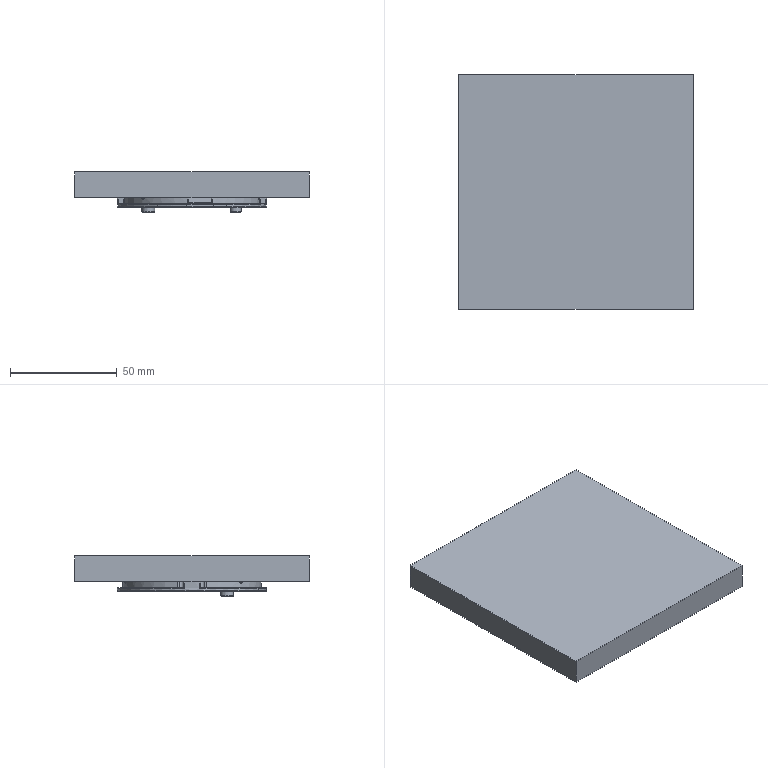NC program | NX | posted with a generic post | part box 110 x 110 x 18.8 mm
Lines 1770 to 3401 of 9447, first 1467 of 1628 lines:
(CAVITY_MILL_COPY_1 , TOOL : D6)
N3532 T16 M6
N3534 G54
N3536 G17 G0 G90 X7.71 Y22.388 S9500 M3
N3538 G43 Z30. H16
N3540 Z-4.5
N3542 G94 G1 Z-5.5 F1000.
N3544 X8.202 Y21.964
N3546 G3 X9.184 Y21.777 R1.
N3548 G2 X10.5 Y22. R4. F1600.
N3550 G1 X16.333
N3552 G3 X9.42 Y25.73 R27.4
N3554 X8.435 Y25.558 R1.
N3556 G1 X7.786 Y25.016
N3558 Z-4.5
N3560 G0 X7.71 Y22.388 Z-5.
N3562 G1 Z-6. F1000.
N3564 X8.202 Y21.964
N3566 G3 X9.184 Y21.777 R1.
N3568 G2 X10.5 Y22. R4. F1600.
N3570 G1 X16.333
N3572 G3 X9.42 Y25.73 R27.4
N3574 X8.435 Y25.558 R1.
N3576 G1 X7.786 Y25.016
N3578 Z-5.
N3580 G0 X7.71 Y22.388 Z-5.5
N3582 G1 Z-6.5 F1000.
N3584 X8.202 Y21.964
N3586 G3 X9.184 Y21.777 R1.
N3588 G2 X10.5 Y22. R4. F1600.
N3590 G1 X16.333
N3592 G3 X9.42 Y25.73 R27.4
N3594 X8.435 Y25.558 R1.
N3596 G1 X7.786 Y25.016
N3598 Z-5.5
N3600 G0 X7.71 Y22.388 Z-6.
N3602 G1 Z-7. F1000.
N3604 X8.202 Y21.964
N3606 G3 X9.184 Y21.777 R1.
N3608 G2 X10.5 Y22. R4. F1600.
N3610 G1 X16.333
N3612 G3 X9.42 Y25.73 R27.4
N3614 X8.435 Y25.558 R1.
N3616 G1 X7.786 Y25.016
N3618 Z-6.
N3620 G0 X7.71 Y22.388 Z-6.5
N3622 G1 Z-7.5 F1000.
N3624 X8.202 Y21.964
N3626 G3 X9.184 Y21.777 R1.
N3628 G2 X10.5 Y22. R4. F1600.
N3630 G1 X16.333
N3632 G3 X9.42 Y25.73 R27.4
N3634 X8.435 Y25.558 R1.
N3636 G1 X7.786 Y25.016
N3638 Z-6.5
N3640 G0 X7.71 Y22.388 Z-7.
N3642 G1 Z-8. F1000.
N3644 X8.202 Y21.964
N3646 G3 X9.184 Y21.777 R1.
N3648 G2 X10.5 Y22. R4. F1600.
N3650 G1 X16.333
N3652 G3 X9.42 Y25.73 R27.4
N3654 X8.435 Y25.558 R1.
N3656 G1 X7.786 Y25.016
N3658 Z-7.
N3660 G0 X7.71 Y22.388 Z-7.5
N3662 G1 Z-8.5 F1000.
N3664 X8.202 Y21.964
N3666 G3 X9.184 Y21.777 R1.
N3668 G2 X10.5 Y22. R4. F1600.
N3670 G1 X16.333
N3672 G3 X9.42 Y25.73 R27.4
N3674 X8.435 Y25.558 R1.
N3676 G1 X7.786 Y25.016
N3678 Z-7.5
N3680 G0 X7.71 Y22.388 Z-8.
N3682 G1 Z-9. F1000.
N3684 X8.202 Y21.964
N3686 G3 X9.184 Y21.777 R1.
N3688 G2 X10.5 Y22. R4. F1600.
N3690 G1 X16.333
N3692 G3 X9.42 Y25.73 R27.4
N3694 X8.435 Y25.558 R1.
N3696 G1 X7.786 Y25.016
N3698 Z-8.
N3700 G0 X7.71 Y22.388 Z-8.5
N3702 G1 Z-9.5 F1000.
N3704 X8.202 Y21.964
N3706 G3 X9.184 Y21.777 R1.
N3708 G2 X10.5 Y22. R4. F1600.
N3710 G1 X16.333
N3712 G3 X9.42 Y25.73 R27.4
N3714 X8.435 Y25.558 R1.
N3716 G1 X7.786 Y25.016
N3718 Z-8.5
N3720 G0 X7.71 Y22.388 Z-9.
N3722 G1 Z-10. F1000.
N3724 X8.202 Y21.964
N3726 G3 X9.184 Y21.777 R1.
N3728 G2 X10.5 Y22. R4. F1600.
N3730 G1 X16.333
N3732 G3 X9.42 Y25.73 R27.4
N3734 X8.435 Y25.558 R1.
N3736 G1 X7.786 Y25.016
N3738 Z-9.
N3740 G0 X7.71 Y22.388 Z-9.5
N3742 G1 Z-10.5 F1000.
N3744 X8.202 Y21.964
N3746 G3 X9.184 Y21.777 R1.
N3748 G2 X10.5 Y22. R4. F1600.
N3750 G1 X16.333
N3752 G3 X9.42 Y25.73 R27.4
N3754 X8.435 Y25.558 R1.
N3756 G1 X7.786 Y25.016
N3758 Z-9.5
N3760 G0 X7.71 Y22.388 Z-10.
N3762 G1 Z-11. F1000.
N3764 X8.202 Y21.964
N3766 G3 X9.184 Y21.777 R1.
N3768 G2 X10.5 Y22. R4. F1600.
N3770 G1 X16.333
N3772 G3 X9.42 Y25.73 R27.4
N3774 X8.435 Y25.558 R1.
N3776 G1 X7.786 Y25.016
N3778 Z-10.
N3780 G0 X7.71 Y22.388 Z-10.5
N3782 G1 Z-11.5 F1000.
N3784 X8.202 Y21.964
N3786 G3 X9.184 Y21.777 R1.
N3788 G2 X10.5 Y22. R4. F1600.
N3790 G1 X16.333
N3792 G3 X9.42 Y25.73 R27.4
N3794 X8.435 Y25.558 R1.
N3796 G1 X7.786 Y25.016
N3798 Z-10.5
N3800 G0 Z30.
N3802 X26.5 Y2.101
N3804 Z2.
N3806 G1 Y-1.733 Z1.799 F1000.
N3808 X26.714 Y-1.548 Z1.784
N3810 X27.121 Y-1.282 Z1.759
N3812 X27.375 Y-1.159 Z1.744
N3814 X27.407 Y-0.419 Z1.705
N3816 X27.381 Y1.261 Z1.617
N3818 X27.252 Y2.937 Z1.529
N3820 X27.021 Y4.602 Z1.441
N3822 X26.688 Y6.249 Z1.353
N3824 X26.5 Y6.965 Z1.314
N3826 Y-1.733 Z0.858
N3828 X26.714 Y-1.548 Z0.843
N3830 X27.121 Y-1.282 Z0.818
N3832 X27.375 Y-1.159 Z0.803
N3834 X27.407 Y-0.419 Z0.764
N3836 X27.381 Y1.261 Z0.676
N3838 X27.252 Y2.937 Z0.588
N3840 X27.021 Y4.602 Z0.5
N3842 X26.688 Y6.249 Z0.412
N3844 X26.5 Y6.965 Z0.373
N3846 Y-1.733 Z-0.083
N3848 X26.714 Y-1.548 Z-0.098
N3850 X27.121 Y-1.282 Z-0.123
N3852 X27.375 Y-1.159 Z-0.138
N3854 X27.407 Y-0.419 Z-0.177
N3856 X27.381 Y1.261 Z-0.265
N3858 X27.252 Y2.937 Z-0.353
N3860 X27.021 Y4.602 Z-0.441
N3862 X26.688 Y6.249 Z-0.529
N3864 X26.5 Y6.965 Z-0.568
N3866 Y-1.733 Z-1.024
N3868 X26.714 Y-1.548 Z-1.038
N3870 X27.121 Y-1.282 Z-1.064
N3872 X27.375 Y-1.159 Z-1.079
N3874 X27.407 Y-0.419 Z-1.117
N3876 X27.381 Y1.261 Z-1.206
N3878 X27.252 Y2.937 Z-1.294
N3880 X27.021 Y4.602 Z-1.382
N3882 X26.688 Y6.249 Z-1.47
N3884 X26.5 Y6.965 Z-1.509
N3886 Y-1.733 Z-1.964
N3888 X26.714 Y-1.548 Z-1.979
N3890 X27.121 Y-1.282 Z-2.005
N3892 X27.375 Y-1.159 Z-2.02
N3894 X27.407 Y-0.419 Z-2.058
N3896 X27.381 Y1.261 Z-2.146
N3898 X27.252 Y2.937 Z-2.235
N3900 X27.021 Y4.602 Z-2.323
N3902 X26.688 Y6.249 Z-2.411
N3904 X26.5 Y6.965 Z-2.449
N3906 Y-1.733 Z-2.905
N3908 X26.714 Y-1.548 Z-2.92
N3910 X27.121 Y-1.282 Z-2.946
N3912 X27.375 Y-1.159 Z-2.96
N3914 X27.407 Y-0.419 Z-2.999
N3916 X27.381 Y1.261 Z-3.087
N3918 X27.252 Y2.937 Z-3.175
N3920 X27.021 Y4.602 Z-3.263
N3922 X26.688 Y6.249 Z-3.352
N3924 X26.5 Y6.965 Z-3.39
N3926 Y-1.733 Z-3.846
N3928 X26.714 Y-1.548 Z-3.861
N3930 X27.121 Y-1.282 Z-3.886
N3932 X27.375 Y-1.159 Z-3.901
N3934 X27.407 Y-0.419 Z-3.94
N3936 X27.381 Y1.261 Z-4.028
N3938 X27.252 Y2.937 Z-4.116
N3940 X27.021 Y4.602 Z-4.204
N3942 X26.688 Y6.249 Z-4.292
N3944 X26.5 Y6.965 Z-4.331
N3946 Y-1.733 Z-4.787
N3948 X26.714 Y-1.548 Z-4.802
N3950 X27.121 Y-1.282 Z-4.827
N3952 X27.375 Y-1.159 Z-4.842
N3954 X27.407 Y-0.419 Z-4.881
N3956 X27.381 Y1.261 Z-4.969
N3958 X27.252 Y2.937 Z-5.057
N3960 X27.021 Y4.602 Z-5.145
N3962 X26.688 Y6.249 Z-5.233
N3964 X26.5 Y6.965 Z-5.272
N3966 Y2.616 Z-5.5
N3968 Y-1.733 F1600.
N3970 G2 X27.375 Y-1.159 R4.
N3972 G3 X26.5 Y6.965 R27.4
N3974 G1 Y2.616
N3976 G3 X27. Y1.75 R1.
N3978 G1 Z-4.5
N3980 G0 X27.389 Y0.724
N3982 G1 X27.381 Y1.261 Z-4.528 F1000.
N3984 X27.252 Y2.937 Z-4.616
N3986 X27.021 Y4.602 Z-4.704
N3988 X26.688 Y6.249 Z-4.792
N3990 X26.5 Y6.965 Z-4.831
N3992 Y-1.733 Z-5.287
N3994 X26.714 Y-1.548 Z-5.302
N3996 X27.121 Y-1.282 Z-5.327
N3998 X27.375 Y-1.159 Z-5.342
N4000 X27.407 Y-0.419 Z-5.381
N4002 X27.381 Y1.261 Z-5.469
N4004 X27.252 Y2.937 Z-5.557
N4006 X27.021 Y4.602 Z-5.645
N4008 X26.688 Y6.249 Z-5.733
N4010 X26.5 Y6.965 Z-5.772
N4012 Y2.616 Z-6.
N4014 Y-1.733 F1600.
N4016 G2 X27.375 Y-1.159 R4.
N4018 G3 X26.5 Y6.965 R27.4
N4020 G1 Y2.616
N4022 G3 X27. Y1.75 R1.
N4024 G1 Z-5.
N4026 G0 X27.389 Y0.724
N4028 G1 X27.381 Y1.261 Z-5.028 F1000.
N4030 X27.252 Y2.937 Z-5.116
N4032 X27.021 Y4.602 Z-5.204
N4034 X26.688 Y6.249 Z-5.292
N4036 X26.5 Y6.965 Z-5.331
N4038 Y-1.733 Z-5.787
N4040 X26.714 Y-1.548 Z-5.802
N4042 X27.121 Y-1.282 Z-5.827
N4044 X27.375 Y-1.159 Z-5.842
N4046 X27.407 Y-0.419 Z-5.881
N4048 X27.381 Y1.261 Z-5.969
N4050 X27.252 Y2.937 Z-6.057
N4052 X27.021 Y4.602 Z-6.145
N4054 X26.688 Y6.249 Z-6.233
N4056 X26.5 Y6.965 Z-6.272
N4058 Y2.616 Z-6.5
N4060 Y-1.733 F1600.
N4062 G2 X27.375 Y-1.159 R4.
N4064 G3 X26.5 Y6.965 R27.4
N4066 G1 Y2.616
N4068 G3 X27. Y1.75 R1.
N4070 G1 Z-5.5
N4072 G0 X27.389 Y0.724
N4074 G1 X27.381 Y1.261 Z-5.528 F1000.
N4076 X27.252 Y2.937 Z-5.616
N4078 X27.021 Y4.602 Z-5.704
N4080 X26.688 Y6.249 Z-5.792
N4082 X26.5 Y6.965 Z-5.831
N4084 Y-1.733 Z-6.287
N4086 X26.714 Y-1.548 Z-6.302
N4088 X27.121 Y-1.282 Z-6.327
N4090 X27.375 Y-1.159 Z-6.342
N4092 X27.407 Y-0.419 Z-6.381
N4094 X27.381 Y1.261 Z-6.469
N4096 X27.252 Y2.937 Z-6.557
N4098 X27.021 Y4.602 Z-6.645
N4100 X26.688 Y6.249 Z-6.733
N4102 X26.5 Y6.965 Z-6.772
N4104 Y2.616 Z-7.
N4106 Y-1.733 F1600.
N4108 G2 X27.375 Y-1.159 R4.
N4110 G3 X26.5 Y6.965 R27.4
N4112 G1 Y2.616
N4114 G3 X27. Y1.75 R1.
N4116 G1 Z-6.
N4118 G0 X27.389 Y0.724
N4120 G1 X27.381 Y1.261 Z-6.028 F1000.
N4122 X27.252 Y2.937 Z-6.116
N4124 X27.021 Y4.602 Z-6.204
N4126 X26.688 Y6.249 Z-6.292
N4128 X26.5 Y6.965 Z-6.331
N4130 Y-1.733 Z-6.787
N4132 X26.714 Y-1.548 Z-6.802
N4134 X27.121 Y-1.282 Z-6.827
N4136 X27.375 Y-1.159 Z-6.842
N4138 X27.407 Y-0.419 Z-6.881
N4140 X27.381 Y1.261 Z-6.969
N4142 X27.252 Y2.937 Z-7.057
N4144 X27.021 Y4.602 Z-7.145
N4146 X26.688 Y6.249 Z-7.233
N4148 X26.5 Y6.965 Z-7.272
N4150 Y2.616 Z-7.5
N4152 Y-1.733 F1600.
N4154 G2 X27.375 Y-1.159 R4.
N4156 G3 X26.5 Y6.965 R27.4
N4158 G1 Y2.616
N4160 G3 X27. Y1.75 R1.
N4162 G1 Z-6.5
N4164 G0 X27.389 Y0.724
N4166 G1 X27.381 Y1.261 Z-6.528 F1000.
N4168 X27.252 Y2.937 Z-6.616
N4170 X27.021 Y4.602 Z-6.704
N4172 X26.688 Y6.249 Z-6.792
N4174 X26.5 Y6.965 Z-6.831
N4176 Y-1.733 Z-7.287
N4178 X26.714 Y-1.548 Z-7.302
N4180 X27.121 Y-1.282 Z-7.327
N4182 X27.375 Y-1.159 Z-7.342
N4184 X27.407 Y-0.419 Z-7.381
N4186 X27.381 Y1.261 Z-7.469
N4188 X27.252 Y2.937 Z-7.557
N4190 X27.021 Y4.602 Z-7.645
N4192 X26.688 Y6.249 Z-7.733
N4194 X26.5 Y6.965 Z-7.772
N4196 Y2.616 Z-8.
N4198 Y-1.733 F1600.
N4200 G2 X27.375 Y-1.159 R4.
N4202 G3 X26.5 Y6.965 R27.4
N4204 G1 Y2.616
N4206 G3 X27. Y1.75 R1.
N4208 G1 Z-7.
N4210 G0 X27.389 Y0.724
N4212 G1 X27.381 Y1.261 Z-7.028 F1000.
N4214 X27.252 Y2.937 Z-7.116
N4216 X27.021 Y4.602 Z-7.204
N4218 X26.688 Y6.249 Z-7.292
N4220 X26.5 Y6.965 Z-7.331
N4222 Y-1.733 Z-7.787
N4224 X26.714 Y-1.548 Z-7.802
N4226 X27.121 Y-1.282 Z-7.827
N4228 X27.375 Y-1.159 Z-7.842
N4230 X27.407 Y-0.419 Z-7.881
N4232 X27.381 Y1.261 Z-7.969
N4234 X27.252 Y2.937 Z-8.057
N4236 X27.021 Y4.602 Z-8.145
N4238 X26.688 Y6.249 Z-8.233
N4240 X26.5 Y6.965 Z-8.272
N4242 Y2.616 Z-8.5
N4244 Y-1.733 F1600.
N4246 G2 X27.375 Y-1.159 R4.
N4248 G3 X26.5 Y6.965 R27.4
N4250 G1 Y2.616
N4252 G3 X27. Y1.75 R1.
N4254 G1 Z-7.5
N4256 G0 X27.389 Y0.724
N4258 G1 X27.381 Y1.261 Z-7.528 F1000.
N4260 X27.252 Y2.937 Z-7.616
N4262 X27.021 Y4.602 Z-7.704
N4264 X26.688 Y6.249 Z-7.792
N4266 X26.5 Y6.965 Z-7.831
N4268 Y-1.733 Z-8.287
N4270 X26.714 Y-1.548 Z-8.302
N4272 X27.121 Y-1.282 Z-8.327
N4274 X27.375 Y-1.159 Z-8.342
N4276 X27.407 Y-0.419 Z-8.381
N4278 X27.381 Y1.261 Z-8.469
N4280 X27.252 Y2.937 Z-8.557
N4282 X27.021 Y4.602 Z-8.645
N4284 X26.688 Y6.249 Z-8.733
N4286 X26.5 Y6.965 Z-8.772
N4288 Y2.616 Z-9.
N4290 Y-1.733 F1600.
N4292 G2 X27.375 Y-1.159 R4.
N4294 G3 X26.5 Y6.965 R27.4
N4296 G1 Y2.616
N4298 G3 X27. Y1.75 R1.
N4300 G1 Z-8.
N4302 G0 X27.389 Y0.724
N4304 G1 X27.381 Y1.261 Z-8.028 F1000.
N4306 X27.252 Y2.937 Z-8.116
N4308 X27.021 Y4.602 Z-8.204
N4310 X26.688 Y6.249 Z-8.292
N4312 X26.5 Y6.965 Z-8.331
N4314 Y-1.733 Z-8.787
N4316 X26.714 Y-1.548 Z-8.802
N4318 X27.121 Y-1.282 Z-8.827
N4320 X27.375 Y-1.159 Z-8.842
N4322 X27.407 Y-0.419 Z-8.881
N4324 X27.381 Y1.261 Z-8.969
N4326 X27.252 Y2.937 Z-9.057
N4328 X27.021 Y4.602 Z-9.145
N4330 X26.688 Y6.249 Z-9.233
N4332 X26.5 Y6.965 Z-9.272
N4334 Y2.616 Z-9.5
N4336 Y-1.733 F1600.
N4338 G2 X27.375 Y-1.159 R4.
N4340 G3 X26.5 Y6.965 R27.4
N4342 G1 Y2.616
N4344 G3 X27. Y1.75 R1.
N4346 G1 Z-8.5
N4348 G0 X27.389 Y0.724
N4350 G1 X27.381 Y1.261 Z-8.528 F1000.
N4352 X27.252 Y2.937 Z-8.616
N4354 X27.021 Y4.602 Z-8.704
N4356 X26.688 Y6.249 Z-8.792
N4358 X26.5 Y6.965 Z-8.831
N4360 Y-1.733 Z-9.287
N4362 X26.714 Y-1.548 Z-9.302
N4364 X27.121 Y-1.282 Z-9.327
N4366 X27.375 Y-1.159 Z-9.342
N4368 X27.407 Y-0.419 Z-9.381
N4370 X27.381 Y1.261 Z-9.469
N4372 X27.252 Y2.937 Z-9.557
N4374 X27.021 Y4.602 Z-9.645
N4376 X26.688 Y6.249 Z-9.733
N4378 X26.5 Y6.965 Z-9.772
N4380 Y2.616 Z-10.
N4382 Y-1.733 F1600.
N4384 G2 X27.375 Y-1.159 R4.
N4386 G3 X26.5 Y6.965 R27.4
N4388 G1 Y2.616
N4390 G3 X27. Y1.75 R1.
N4392 G1 Z-9.
N4394 G0 X27.389 Y0.724
N4396 G1 X27.381 Y1.261 Z-9.028 F1000.
N4398 X27.252 Y2.937 Z-9.116
N4400 X27.021 Y4.602 Z-9.204
N4402 X26.688 Y6.249 Z-9.292
N4404 X26.5 Y6.965 Z-9.331
N4406 Y-1.733 Z-9.787
N4408 X26.714 Y-1.548 Z-9.802
N4410 X27.121 Y-1.282 Z-9.827
N4412 X27.375 Y-1.159 Z-9.842
N4414 X27.407 Y-0.419 Z-9.881
N4416 X27.381 Y1.261 Z-9.969
N4418 X27.252 Y2.937 Z-10.057
N4420 X27.021 Y4.602 Z-10.145
N4422 X26.688 Y6.249 Z-10.233
N4424 X26.5 Y6.965 Z-10.272
N4426 Y2.616 Z-10.5
N4428 Y-1.733 F1600.
N4430 G2 X27.375 Y-1.159 R4.
N4432 G3 X26.5 Y6.965 R27.4
N4434 G1 Y2.616
N4436 G3 X27. Y1.75 R1.
N4438 G1 Z-9.5
N4440 G0 X27.389 Y0.724
N4442 G1 X27.381 Y1.261 Z-9.528 F1000.
N4444 X27.252 Y2.937 Z-9.616
N4446 X27.021 Y4.602 Z-9.704
N4448 X26.688 Y6.249 Z-9.792
N4450 X26.5 Y6.965 Z-9.831
N4452 Y-1.733 Z-10.287
N4454 X26.714 Y-1.548 Z-10.302
N4456 X27.121 Y-1.282 Z-10.327
N4458 X27.375 Y-1.159 Z-10.342
N4460 X27.407 Y-0.419 Z-10.381
N4462 X27.381 Y1.261 Z-10.469
N4464 X27.252 Y2.937 Z-10.557
N4466 X27.021 Y4.602 Z-10.645
N4468 X26.688 Y6.249 Z-10.733
N4470 X26.5 Y6.965 Z-10.772
N4472 Y2.616 Z-11.
N4474 Y-1.733 F1600.
N4476 G2 X27.375 Y-1.159 R4.
N4478 G3 X26.5 Y6.965 R27.4
N4480 G1 Y2.616
N4482 G3 X27. Y1.75 R1.
N4484 G1 Z-10.
N4486 G0 X27.389 Y0.724
N4488 G1 X27.381 Y1.261 Z-10.028 F1000.
N4490 X27.252 Y2.937 Z-10.116
N4492 X27.021 Y4.602 Z-10.204
N4494 X26.688 Y6.249 Z-10.292
N4496 X26.5 Y6.965 Z-10.331
N4498 Y-1.733 Z-10.787
N4500 X26.714 Y-1.548 Z-10.802
N4502 X27.121 Y-1.282 Z-10.827
N4504 X27.375 Y-1.159 Z-10.842
N4506 X27.407 Y-0.419 Z-10.881
N4508 X27.381 Y1.261 Z-10.969
N4510 X27.252 Y2.937 Z-11.057
N4512 X27.021 Y4.602 Z-11.145
N4514 X26.688 Y6.249 Z-11.233
N4516 X26.5 Y6.965 Z-11.272
N4518 Y2.616 Z-11.5
N4520 Y-1.733 F1600.
N4522 G2 X27.375 Y-1.159 R4.
N4524 G3 X26.5 Y6.965 R27.4
N4526 G1 Y2.616
N4528 G3 X27. Y1.75 R1.
N4530 G1 Z-10.5
N4532 G0 Z30.
N4534 X35.854 Y7.345
N4536 Z-4.5
N4538 G1 Z-5.5 F1000.
N4540 X35.276 Y7.05
N4542 G3 X34.733 Y6.21 R1.
N4544 G2 X34.602 Y5.381 R4. F1600.
N4546 X34.978 Y4.631 R4.
N4548 G3 X35.751 Y3.996 R1.
N4550 G1 X36.391 Y3.89
N4552 Z-4.5
N4554 G0 X35.854 Y7.345 Z-5.
N4556 G1 Z-6. F1000.
N4558 X35.276 Y7.05
N4560 G3 X34.733 Y6.21 R1.
N4562 G2 X34.602 Y5.381 R4. F1600.
N4564 X34.978 Y4.63 R4.
N4566 G3 X35.751 Y3.996 R1.
N4568 G1 X36.391 Y3.89
N4570 Z-5.
N4572 G0 X35.854 Y7.345 Z-5.5
N4574 G1 Z-6.5 F1000.
N4576 X35.276 Y7.05
N4578 G3 X34.733 Y6.21 R1.
N4580 G2 X34.602 Y5.381 R4. F1600.
N4582 X34.978 Y4.63 R4.
N4584 G3 X35.751 Y3.996 R1.
N4586 G1 X36.391 Y3.89
N4588 Z-5.5
N4590 G0 X35.854 Y7.345 Z-6.
N4592 G1 Z-7. F1000.
N4594 X35.276 Y7.05
N4596 G3 X34.733 Y6.21 R1.
N4598 G2 X34.602 Y5.381 R4. F1600.
N4600 X34.978 Y4.631 R4.
N4602 G3 X35.751 Y3.996 R1.
N4604 G1 X36.391 Y3.89
N4606 Z-6.
N4608 G0 X35.854 Y7.345 Z-6.5
N4610 G1 Z-7.5 F1000.
N4612 X35.276 Y7.05
N4614 G3 X34.733 Y6.21 R1.
N4616 G2 X34.602 Y5.381 R4. F1600.
N4618 X34.978 Y4.631 R4.
N4620 G3 X35.751 Y3.996 R1.
N4622 G1 X36.391 Y3.89
N4624 Z-6.5
N4626 G0 X35.854 Y7.345 Z-7.
N4628 G1 Z-8. F1000.
N4630 X35.276 Y7.05
N4632 G3 X34.733 Y6.21 R1.
N4634 G2 X34.602 Y5.381 R4. F1600.
N4636 X34.978 Y4.631 R4.
N4638 G3 X35.751 Y3.996 R1.
N4640 G1 X36.391 Y3.89
N4642 Z-7.
N4644 G0 X35.854 Y7.345 Z-7.5
N4646 G1 Z-8.5 F1000.
N4648 X35.276 Y7.05
N4650 G3 X34.733 Y6.21 R1.
N4652 G2 X34.602 Y5.381 R4. F1600.
N4654 X34.978 Y4.63 R4.
N4656 G3 X35.751 Y3.996 R1.
N4658 G1 X36.391 Y3.89
N4660 Z-7.5
N4662 G0 X35.854 Y7.345 Z-8.
N4664 G1 Z-9. F1000.
N4666 X35.276 Y7.05
N4668 G3 X34.733 Y6.21 R1.
N4670 G2 X34.602 Y5.381 R4. F1600.
N4672 X34.978 Y4.63 R4.
N4674 G3 X35.751 Y3.996 R1.
N4676 G1 X36.391 Y3.89
N4678 Z-8.
N4680 G0 X35.249 Y9.851 Z-8.5
N4682 G1 Z-9.5 F1000.
N4684 X34.682 Y9.311
N4686 G3 X34.401 Y8.351 R1.
N4688 G2 X34.705 Y6.979 R35.4 F1600.
N4690 X35.894 Y6.627 R3.5
N4692 G3 X36.892 Y6.685 R1.
N4694 G1 X37.421 Y7.033
N4696 Z-8.5
N4698 G0 X35.249 Y9.851 Z-9.
N4700 G1 Z-10. F1000.
N4702 X34.682 Y9.311
N4704 G3 X34.401 Y8.351 R1.
N4706 G2 X34.705 Y6.979 R35.4 F1600.
N4708 X35.894 Y6.627 R3.5
N4710 G3 X36.892 Y6.685 R1.
N4712 G1 X37.421 Y7.033
N4714 Z-9.
N4716 G0 X35.249 Y9.851 Z-9.5
N4718 G1 Z-10.5 F1000.
N4720 X34.682 Y9.311
N4722 G3 X34.401 Y8.351 R1.
N4724 G2 X34.705 Y6.979 R35.4 F1600.
N4726 X35.894 Y6.627 R3.5
N4728 G3 X36.892 Y6.685 R1.
N4730 G1 X37.421 Y7.033
N4732 Z-9.5
N4734 G0 X35.249 Y9.851 Z-10.
N4736 G1 Z-11. F1000.
N4738 X34.682 Y9.311
N4740 G3 X34.401 Y8.351 R1.
N4742 G2 X34.705 Y6.979 R35.4 F1600.
N4744 X35.894 Y6.627 R3.5
N4746 G3 X36.892 Y6.685 R1.
N4748 G1 X37.421 Y7.033
N4750 Z-10.
N4752 G0 X35.249 Y9.851 Z-10.5
N4754 G1 Z-11.5 F1000.
N4756 X34.682 Y9.311
N4758 G3 X34.401 Y8.351 R1.
N4760 G2 X34.705 Y6.979 R35.4 F1600.
N4762 X35.894 Y6.627 R3.5
N4764 G3 X36.892 Y6.685 R1.
N4766 G1 X37.421 Y7.033
N4768 Z-10.5
N4770 G0 X35.249 Y9.851 Z-11.
N4772 G1 Z-12. F1000.
N4774 X34.682 Y9.311
N4776 G3 X34.401 Y8.351 R1.
N4778 G2 X34.705 Y6.979 R35.4 F1600.
N4780 X35.894 Y6.627 R3.5
N4782 G3 X36.892 Y6.685 R1.
N4784 G1 X37.421 Y7.033
N4786 Z-11.
N4788 G0 Z30.
N4790 X36.391 Y-3.89
N4792 Z-4.5
N4794 G1 Z-5.5 F1000.
N4796 X35.751 Y-3.996
N4798 G3 X34.978 Y-4.631 R1.
N4800 G2 X34.602 Y-5.381 R4. F1600.
N4802 X34.733 Y-6.21 R4.
N4804 G3 X35.276 Y-7.05 R1.
N4806 G1 X35.854 Y-7.345
N4808 Z-4.5
N4810 G0 X36.391 Y-3.89 Z-5.
N4812 G1 Z-6. F1000.
N4814 X35.751 Y-3.996
N4816 G3 X34.978 Y-4.631 R1.
N4818 G2 X34.602 Y-5.381 R4. F1600.
N4820 X34.733 Y-6.21 R4.
N4822 G3 X35.276 Y-7.05 R1.
N4824 G1 X35.854 Y-7.345
N4826 Z-5.
N4828 G0 X36.391 Y-3.89 Z-5.5
N4830 G1 Z-6.5 F1000.
N4832 X35.751 Y-3.996
N4834 G3 X34.978 Y-4.631 R1.
N4836 G2 X34.602 Y-5.381 R4. F1600.
N4838 X34.733 Y-6.21 R4.
N4840 G3 X35.276 Y-7.05 R1.
N4842 G1 X35.854 Y-7.345
N4844 Z-5.5
N4846 G0 X36.391 Y-3.89 Z-6.
N4848 G1 Z-7. F1000.
N4850 X35.751 Y-3.996
N4852 G3 X34.978 Y-4.631 R1.
N4854 G2 X34.602 Y-5.381 R4. F1600.
N4856 X34.733 Y-6.21 R4.
N4858 G3 X35.276 Y-7.05 R1.
N4860 G1 X35.854 Y-7.345
N4862 Z-6.
N4864 G0 X36.391 Y-3.89 Z-6.5
N4866 G1 Z-7.5 F1000.
N4868 X35.751 Y-3.996
N4870 G3 X34.978 Y-4.631 R1.
N4872 G2 X34.602 Y-5.381 R4. F1600.
N4874 X34.733 Y-6.21 R4.
N4876 G3 X35.276 Y-7.05 R1.
N4878 G1 X35.854 Y-7.345
N4880 Z-6.5
N4882 G0 X36.391 Y-3.89 Z-7.
N4884 G1 Z-8. F1000.
N4886 X35.751 Y-3.996
N4888 G3 X34.978 Y-4.631 R1.
N4890 G2 X34.602 Y-5.381 R4. F1600.
N4892 X34.733 Y-6.21 R4.
N4894 G3 X35.276 Y-7.05 R1.
N4896 G1 X35.854 Y-7.345
N4898 Z-7.
N4900 G0 X36.391 Y-3.89 Z-7.5
N4902 G1 Z-8.5 F1000.
N4904 X35.751 Y-3.996
N4906 G3 X34.978 Y-4.631 R1.
N4908 G2 X34.602 Y-5.381 R4. F1600.
N4910 X34.733 Y-6.21 R4.
N4912 G3 X35.276 Y-7.05 R1.
N4914 G1 X35.854 Y-7.345
N4916 Z-7.5
N4918 G0 X36.391 Y-3.89 Z-8.
N4920 G1 Z-9. F1000.
N4922 X35.751 Y-3.996
N4924 G3 X34.978 Y-4.631 R1.
N4926 G2 X34.602 Y-5.381 R4. F1600.
N4928 X34.733 Y-6.21 R4.
N4930 G3 X35.276 Y-7.05 R1.
N4932 G1 X35.854 Y-7.345
N4934 Z-8.
N4936 G0 X37.421 Y-7.033 Z-8.5
N4938 G1 Z-9.5 F1000.
N4940 X36.892 Y-6.685
N4942 G3 X35.894 Y-6.627 R1.
N4944 G2 X34.698 Y-6.98 R3.5 F1600.
N4946 X34.654 Y-7.231 R4.
N4948 X34.401 Y-8.351 R35.4
N4950 G3 X34.682 Y-9.311 R1.
N4952 G1 X35.249 Y-9.851
N4954 Z-8.5
N4956 G0 X37.421 Y-7.033 Z-9.
N4958 G1 Z-10. F1000.
N4960 X36.892 Y-6.685
N4962 G3 X35.894 Y-6.627 R1.
N4964 G2 X34.698 Y-6.98 R3.5 F1600.
N4966 X34.654 Y-7.231 R4.
N4968 X34.401 Y-8.351 R35.4
N4970 G3 X34.682 Y-9.311 R1.
N4972 G1 X35.249 Y-9.851
N4974 Z-9.
N4976 G0 X37.421 Y-7.033 Z-9.5
N4978 G1 Z-10.5 F1000.
N4980 X36.892 Y-6.685
N4982 G3 X35.894 Y-6.627 R1.
N4984 G2 X34.698 Y-6.98 R3.5 F1600.
N4986 X34.654 Y-7.231 R4.
N4988 X34.401 Y-8.351 R35.4
N4990 G3 X34.682 Y-9.311 R1.
N4992 G1 X35.249 Y-9.851
N4994 Z-9.5
N4996 G0 X37.421 Y-7.033 Z-10.
N4998 G1 Z-11. F1000.
N5000 X36.892 Y-6.685
N5002 G3 X35.894 Y-6.627 R1.
N5004 G2 X34.698 Y-6.98 R3.5 F1600.
N5006 X34.654 Y-7.231 R4.
N5008 X34.401 Y-8.351 R35.4
N5010 G3 X34.682 Y-9.311 R1.
N5012 G1 X35.249 Y-9.851
N5014 Z-10.
N5016 G0 X37.421 Y-7.033 Z-10.5
N5018 G1 Z-11.5 F1000.
N5020 X36.892 Y-6.685
N5022 G3 X35.894 Y-6.627 R1.
N5024 G2 X34.698 Y-6.98 R3.5 F1600.
N5026 X34.654 Y-7.231 R4.
N5028 X34.401 Y-8.351 R35.4
N5030 G3 X34.682 Y-9.311 R1.
N5032 G1 X35.249 Y-9.851
N5034 Z-10.5
N5036 G0 X37.421 Y-7.033 Z-11.
N5038 G1 Z-12. F1000.
N5040 X36.892 Y-6.685
N5042 G3 X35.894 Y-6.627 R1.
N5044 G2 X34.698 Y-6.98 R3.5 F1600.
N5046 X34.654 Y-7.231 R4.
N5048 X34.401 Y-8.351 R35.4
N5050 G3 X34.682 Y-9.311 R1.
N5052 G1 X35.249 Y-9.851
N5054 Z-11.
N5056 G0 Z30.
N5058 X11.227 Y-25.849
N5060 Z-4.5
N5062 G1 Z-5.5 F1000.
N5064 X11.856 Y-25.767
N5066 G3 X12.65 Y-25.16 R1.
N5068 G2 X14.082 Y-23.504 R3.5 F1600.
N5070 G3 X16.333 Y-22. R27.4
N5072 G1 X10.769
N5074 G3 X9.903 Y-22.5 R1.
N5076 G1 X9.549 Y-23.112
N5078 Z-4.5
N5080 G0 X11.227 Y-25.849 Z-5.
N5082 G1 Z-6. F1000.
N5084 X11.856 Y-25.767
N5086 G3 X12.65 Y-25.16 R1.
N5088 G2 X14.082 Y-23.504 R3.5 F1600.
N5090 G3 X16.333 Y-22. R27.4
N5092 G1 X10.769
N5094 G3 X9.903 Y-22.5 R1.
N5096 G1 X9.549 Y-23.112
N5098 Z-5.
N5100 G0 X11.227 Y-25.849 Z-5.5
N5102 G1 Z-6.5 F1000.
N5104 X11.856 Y-25.767
N5106 G3 X12.65 Y-25.16 R1.
N5108 G2 X14.082 Y-23.504 R3.5 F1600.
N5110 G3 X16.333 Y-22. R27.4
N5112 G1 X10.769
N5114 G3 X9.903 Y-22.5 R1.
N5116 G1 X9.549 Y-23.112
N5118 Z-5.5
N5120 G0 X11.227 Y-25.849 Z-6.
N5122 G1 Z-7. F1000.
N5124 X11.856 Y-25.767
N5126 G3 X12.65 Y-25.16 R1.
N5128 G2 X14.082 Y-23.504 R3.5 F1600.
N5130 G3 X16.333 Y-22. R27.4
N5132 G1 X10.769
N5134 G3 X9.903 Y-22.5 R1.
N5136 G1 X9.549 Y-23.112
N5138 Z-6.
N5140 G0 X11.227 Y-25.849 Z-6.5
N5142 G1 Z-7.5 F1000.
N5144 X11.856 Y-25.767
N5146 G3 X12.65 Y-25.16 R1.
N5148 G2 X14.082 Y-23.504 R3.5 F1600.
N5150 G3 X16.333 Y-22. R27.4
N5152 G1 X10.769
N5154 G3 X9.903 Y-22.5 R1.
N5156 G1 X9.549 Y-23.112
N5158 Z-6.5
N5160 G0 X11.227 Y-25.849 Z-7.
N5162 G1 Z-8. F1000.
N5164 X11.856 Y-25.767
N5166 G3 X12.65 Y-25.16 R1.
N5168 G2 X14.082 Y-23.504 R3.5 F1600.
N5170 G3 X16.333 Y-22. R27.4
N5172 G1 X10.769
N5174 G3 X9.903 Y-22.5 R1.
N5176 G1 X9.549 Y-23.112
N5178 Z-7.
N5180 G0 X11.227 Y-25.849 Z-7.5
N5182 G1 Z-8.5 F1000.
N5184 X11.856 Y-25.767
N5186 G3 X12.65 Y-25.16 R1.
N5188 G2 X14.082 Y-23.504 R3.5 F1600.
N5190 G3 X16.333 Y-22. R27.4
N5192 G1 X10.769
N5194 G3 X9.903 Y-22.5 R1.
N5196 G1 X9.549 Y-23.112
N5198 Z-7.5
N5200 G0 X11.227 Y-25.849 Z-8.
N5202 G1 Z-9. F1000.
N5204 X11.856 Y-25.767
N5206 G3 X12.65 Y-25.16 R1.
N5208 G2 X14.082 Y-23.504 R3.5 F1600.
N5210 G3 X16.333 Y-22. R27.4
N5212 G1 X10.769
N5214 G3 X9.903 Y-22.5 R1.
N5216 G1 X9.549 Y-23.112
N5218 Z-8.
N5220 G0 X7.795 Y-25.024 Z-8.5
N5222 G1 Z-9.5 F1000.
N5224 X8.435 Y-25.558
N5226 G3 X9.42 Y-25.73 R1.
N5228 X16.333 Y-22. R27.4 F1600.
N5230 G1 X10.5
N5232 G2 X9.184 Y-21.777 R4.
N5234 G3 X8.202 Y-21.964 R1.
N5236 G1 X7.71 Y-22.388
N5238 Z-8.5
N5240 G0 X7.795 Y-25.024 Z-9.
N5242 G1 Z-10. F1000.
N5244 X8.435 Y-25.558
N5246 G3 X9.42 Y-25.73 R1.
N5248 X16.333 Y-22. R27.4 F1600.
N5250 G1 X10.5
N5252 G2 X9.184 Y-21.777 R4.
N5254 G3 X8.202 Y-21.964 R1.
N5256 G1 X7.71 Y-22.388
N5258 Z-9.
N5260 G0 X7.795 Y-25.024 Z-9.5
N5262 G1 Z-10.5 F1000.
N5264 X8.435 Y-25.558
N5266 G3 X9.42 Y-25.73 R1.
N5268 X16.333 Y-22. R27.4 F1600.
N5270 G1 X10.5
N5272 G2 X9.184 Y-21.777 R4.
N5274 G3 X8.202 Y-21.964 R1.
N5276 G1 X7.71 Y-22.388
N5278 Z-9.5
N5280 G0 X7.795 Y-25.024 Z-10.
N5282 G1 Z-11. F1000.
N5284 X8.435 Y-25.558
N5286 G3 X9.42 Y-25.73 R1.
N5288 X16.333 Y-22. R27.4 F1600.
N5290 G1 X10.5
N5292 G2 X9.184 Y-21.777 R4.
N5294 G3 X8.202 Y-21.964 R1.
N5296 G1 X7.71 Y-22.388
N5298 Z-10.
N5300 G0 X7.795 Y-25.024 Z-10.5
N5302 G1 Z-11.5 F1000.
N5304 X8.435 Y-25.558
N5306 G3 X9.42 Y-25.73 R1.
N5308 X16.333 Y-22. R27.4 F1600.
N5310 G1 X10.5
N5312 G2 X9.184 Y-21.777 R4.
N5314 G3 X8.202 Y-21.964 R1.
N5316 G1 X7.71 Y-22.388
N5318 Z-10.5
N5320 G0 X5.822 Y-24.154 Z-11.
N5322 G1 Z-12. F1000.
N5324 X6.432 Y-24.374
N5326 G3 X7.417 Y-24.196 R1.
N5328 G2 X10. Y-23.25 R4. F1600.
N5330 G1 X10.75
N5332 G3 X12.604 Y-22. R2.
N5334 G1 X10.5
N5336 G2 X7.601 Y-20.756 R4.
N5338 G3 X6.642 Y-20.472 R1.
N5340 G1 X6.011 Y-20.624
N5342 Z-11.
N5344 G0 Z30.
N5346 X5.3 Y-13.24
N5348 Z-11.
N5350 G1 Z-12. F1000.
N5352 X6. Y-12.836
N5354 G3 X6.5 Y-11.97 R1.
N5356 G1 Y-9.75 F1600.
N5358 X4.283
N5360 G3 X3.417 Y-10.25 R1.
N5362 G1 X3.013 Y-10.95
N5364 Z-11.
N5366 G0 Z30.
N5368 X-13.98 Y-20.608
N5370 Z-4.5
N5372 G1 Z-5.5 F1000.
N5374 X-14.461 Y-21.043
N5376 G3 X-14.769 Y-21.995 R1.
N5378 G2 X-14.691 Y-23.129 R4. F1600.
N5380 G3 X-13.567 Y-23.805 R27.4
N5382 X-12.567 Y-23.8 R1.
N5384 G1 X-11.838 Y-23.373
N5386 Z-4.5
N5388 G0 X-13.98 Y-20.608 Z-5.
N5390 G1 Z-6. F1000.
N5392 X-14.461 Y-21.043
N5394 G3 X-14.769 Y-21.994 R1.
N5396 G2 X-14.691 Y-23.129 R4. F1600.
N5398 G3 X-13.567 Y-23.805 R27.4
N5400 X-12.567 Y-23.8 R1.
N5402 G1 X-11.838 Y-23.373
N5404 Z-5.
N5406 G0 X-13.98 Y-20.608 Z-5.5
N5408 G1 Z-6.5 F1000.
N5410 X-14.461 Y-21.043
N5412 G3 X-14.769 Y-21.994 R1.
N5414 G2 X-14.691 Y-23.129 R4. F1600.
N5416 G3 X-13.567 Y-23.805 R27.4
N5418 X-12.567 Y-23.8 R1.
N5420 G1 X-11.838 Y-23.373
N5422 Z-5.5
N5424 G0 X-13.98 Y-20.608 Z-6.
N5426 G1 Z-7. F1000.
N5428 X-14.461 Y-21.043
N5430 G3 X-14.769 Y-21.994 R1.
N5432 G2 X-14.691 Y-23.129 R4. F1600.
N5434 G3 X-13.567 Y-23.805 R27.4
N5436 X-12.567 Y-23.8 R1.
N5438 G1 X-11.838 Y-23.373
N5440 Z-6.
N5442 G0 X-13.98 Y-20.608 Z-6.5
N5444 G1 Z-7.5 F1000.
N5446 X-14.461 Y-21.043
N5448 G3 X-14.769 Y-21.995 R1.
N5450 G2 X-14.691 Y-23.129 R4. F1600.
N5452 G3 X-13.567 Y-23.805 R27.4
N5454 X-12.567 Y-23.8 R1.
N5456 G1 X-11.838 Y-23.373
N5458 Z-6.5
N5460 G0 X-13.98 Y-20.608 Z-7.
N5462 G1 Z-8. F1000.
N5464 X-14.461 Y-21.043
N5466 G3 X-14.769 Y-21.995 R1.
N5468 G2 X-14.691 Y-23.129 R4. F1600.
N5470 G3 X-13.567 Y-23.805 R27.4
N5472 X-12.567 Y-23.8 R1.
N5474 G1 X-11.838 Y-23.373
N5476 Z-7.
N5478 G0 X-13.98 Y-20.608 Z-7.5
N5480 G1 Z-8.5 F1000.
N5482 X-14.461 Y-21.043
N5484 G3 X-14.769 Y-21.995 R1.
N5486 G2 X-14.691 Y-23.129 R4. F1600.
N5488 G3 X-13.567 Y-23.805 R27.4
N5490 X-12.567 Y-23.8 R1.
N5492 G1 X-11.838 Y-23.373
N5494 Z-7.5
N5496 G0 X-13.98 Y-20.608 Z-8.
N5498 G1 Z-9. F1000.
N5500 X-14.461 Y-21.043
N5502 G3 X-14.769 Y-21.995 R1.
N5504 G2 X-14.691 Y-23.129 R4. F1600.
N5506 G3 X-13.567 Y-23.805 R27.4
N5508 X-12.567 Y-23.8 R1.
N5510 G1 X-11.838 Y-23.373
N5512 Z-8.
N5514 G0 X-13.98 Y-20.608 Z-8.5
N5516 G1 Z-9.5 F1000.
N5518 X-14.461 Y-21.043
N5520 G3 X-14.769 Y-21.995 R1.
N5522 G2 X-14.691 Y-23.129 R4. F1600.
N5524 G3 X-13.567 Y-23.805 R27.4
N5526 X-12.567 Y-23.8 R1.
N5528 G1 X-11.838 Y-23.373
N5530 Z-8.5
N5532 G0 X-13.98 Y-20.608 Z-9.
N5534 G1 Z-10. F1000.
N5536 X-14.461 Y-21.043
N5538 G3 X-14.769 Y-21.995 R1.
N5540 G2 X-14.691 Y-23.129 R4. F1600.
N5542 G3 X-13.567 Y-23.805 R27.4
N5544 X-12.567 Y-23.8 R1.
N5546 G1 X-11.838 Y-23.373
N5548 Z-9.
N5550 G0 X-13.98 Y-20.608 Z-9.5
N5552 G1 Z-10.5 F1000.
N5554 X-14.461 Y-21.043
N5556 G3 X-14.769 Y-21.995 R1.
N5558 G2 X-14.691 Y-23.129 R4. F1600.
N5560 G3 X-13.567 Y-23.805 R27.4
N5562 X-12.567 Y-23.8 R1.
N5564 G1 X-11.838 Y-23.373
N5566 Z-9.5
N5568 G0 X-13.98 Y-20.608 Z-10.
N5570 G1 Z-11. F1000.
N5572 X-14.461 Y-21.043
N5574 G3 X-14.769 Y-21.995 R1.
N5576 G2 X-14.691 Y-23.129 R4. F1600.
N5578 G3 X-13.567 Y-23.805 R27.4
N5580 X-12.567 Y-23.8 R1.
N5582 G1 X-11.838 Y-23.373
N5584 Z-10.
N5586 G0 X-13.98 Y-20.608 Z-10.5
N5588 G1 Z-11.5 F1000.
N5590 X-14.461 Y-21.043
N5592 G3 X-14.769 Y-21.994 R1.
N5594 G2 X-14.691 Y-23.129 R4. F1600.
N5596 G3 X-13.567 Y-23.805 R27.4
N5598 X-12.567 Y-23.8 R1.
N5600 G1 X-11.838 Y-23.373
N5602 Z-10.5
N5604 G0 Z30.
N5606 X-23.373 Y-11.838
N5608 Z-4.5
N5610 G1 Z-5.5 F1000.
N5612 X-23.8 Y-12.567
N5614 G3 X-23.805 Y-13.567 R1.
N5616 X-23.129 Y-14.691 R27.4 F1600.
N5618 G2 X-21.995 Y-14.769 R4.
N5620 G3 X-21.043 Y-14.461 R1.
N5622 G1 X-20.608 Y-13.98
N5624 Z-4.5
N5626 G0 X-23.373 Y-11.838 Z-5.
N5628 G1 Z-6. F1000.
N5630 X-23.8 Y-12.567
N5632 G3 X-23.805 Y-13.567 R1.
N5634 X-23.129 Y-14.691 R27.4 F1600.
N5636 G2 X-21.995 Y-14.769 R4.
N5638 G3 X-21.043 Y-14.461 R1.
N5640 G1 X-20.608 Y-13.98
N5642 Z-5.
N5644 G0 X-23.373 Y-11.838 Z-5.5
N5646 G1 Z-6.5 F1000.
N5648 X-23.8 Y-12.567
N5650 G3 X-23.805 Y-13.567 R1.
N5652 X-23.129 Y-14.691 R27.4 F1600.
N5654 G2 X-21.995 Y-14.769 R4.
N5656 G3 X-21.043 Y-14.461 R1.
N5658 G1 X-20.608 Y-13.98
N5660 Z-5.5
N5662 G0 X-23.373 Y-11.838 Z-6.
N5664 G1 Z-7. F1000.
N5666 X-23.8 Y-12.567
N5668 G3 X-23.805 Y-13.567 R1.
N5670 X-23.129 Y-14.691 R27.4 F1600.
N5672 G2 X-21.995 Y-14.769 R4.
N5674 G3 X-21.043 Y-14.461 R1.
N5676 G1 X-20.608 Y-13.98
N5678 Z-6.
N5680 G0 X-23.373 Y-11.838 Z-6.5
N5682 G1 Z-7.5 F1000.
N5684 X-23.8 Y-12.567
N5686 G3 X-23.805 Y-13.567 R1.
N5688 X-23.129 Y-14.691 R27.4 F1600.
N5690 G2 X-21.995 Y-14.769 R4.
N5692 G3 X-21.043 Y-14.461 R1.
N5694 G1 X-20.608 Y-13.98
N5696 Z-6.5
N5698 G0 X-23.373 Y-11.838 Z-7.
N5700 G1 Z-8. F1000.
N5702 X-23.8 Y-12.567
N5704 G3 X-23.805 Y-13.567 R1.
N5706 X-23.129 Y-14.691 R27.4 F1600.
N5708 G2 X-21.995 Y-14.769 R4.
N5710 G3 X-21.043 Y-14.461 R1.
N5712 G1 X-20.608 Y-13.98
N5714 Z-7.
N5716 G0 X-23.373 Y-11.838 Z-7.5
N5718 G1 Z-8.5 F1000.
N5720 X-23.8 Y-12.567
N5722 G3 X-23.805 Y-13.567 R1.
N5724 X-23.129 Y-14.691 R27.4 F1600.
N5726 G2 X-21.995 Y-14.769 R4.
N5728 G3 X-21.043 Y-14.461 R1.
N5730 G1 X-20.608 Y-13.98
N5732 Z-7.5
N5734 G0 X-23.373 Y-11.838 Z-8.
N5736 G1 Z-9. F1000.
N5738 X-23.8 Y-12.567
N5740 G3 X-23.805 Y-13.567 R1.
N5742 X-23.129 Y-14.691 R27.4 F1600.
N5744 G2 X-21.995 Y-14.769 R4.
N5746 G3 X-21.043 Y-14.461 R1.
N5748 G1 X-20.608 Y-13.98
N5750 Z-8.
N5752 G0 X-23.373 Y-11.838 Z-8.5
N5754 G1 Z-9.5 F1000.
N5756 X-23.8 Y-12.567
N5758 G3 X-23.805 Y-13.567 R1.
N5760 X-23.129 Y-14.691 R27.4 F1600.
N5762 G2 X-21.995 Y-14.769 R4.
N5764 G3 X-21.043 Y-14.461 R1.
N5766 G1 X-20.608 Y-13.98
N5768 Z-8.5
N5770 G0 X-23.373 Y-11.838 Z-9.
N5772 G1 Z-10. F1000.
N5774 X-23.8 Y-12.567
N5776 G3 X-23.805 Y-13.567 R1.
N5778 X-23.129 Y-14.691 R27.4 F1600.
N5780 G2 X-21.995 Y-14.769 R4.
N5782 G3 X-21.043 Y-14.461 R1.
N5784 G1 X-20.608 Y-13.98
N5786 Z-9.
N5788 G0 X-23.373 Y-11.838 Z-9.5
N5790 G1 Z-10.5 F1000.
N5792 X-23.8 Y-12.567
N5794 G3 X-23.805 Y-13.567 R1.
N5796 X-23.129 Y-14.691 R27.4 F1600.
N5798 G2 X-21.995 Y-14.769 R4.
N5800 G3 X-21.043 Y-14.461 R1.
N5802 G1 X-20.608 Y-13.98
N5804 Z-9.5
N5806 G0 X-23.373 Y-11.838 Z-10.
N5808 G1 Z-11. F1000.
N5810 X-23.8 Y-12.567
N5812 G3 X-23.805 Y-13.567 R1.
N5814 X-23.129 Y-14.691 R27.4 F1600.
N5816 G2 X-21.995 Y-14.769 R4.
N5818 G3 X-21.043 Y-14.461 R1.
N5820 G1 X-20.608 Y-13.98
N5822 Z-10.
N5824 G0 X-23.373 Y-11.838 Z-10.5
N5826 G1 Z-11.5 F1000.
N5828 X-23.8 Y-12.567
N5830 G3 X-23.805 Y-13.567 R1.
N5832 X-23.129 Y-14.691 R27.4 F1600.
N5834 G2 X-21.995 Y-14.769 R4.
N5836 G3 X-21.043 Y-14.461 R1.
N5838 G1 X-20.608 Y-13.98
N5840 Z-10.5
N5842 G0 Z30.
N5844 X-35.854 Y-7.345
N5846 Z-4.5
N5848 G1 Z-5.5 F1000.
N5850 X-35.276 Y-7.05
N5852 G3 X-34.733 Y-6.21 R1.
N5854 G2 X-34.602 Y-5.381 R4. F1600.
N5856 X-34.978 Y-4.631 R4.
N5858 G3 X-35.751 Y-3.996 R1.
N5860 G1 X-36.391 Y-3.89
N5862 Z-4.5
N5864 G0 X-35.854 Y-7.345 Z-5.
N5866 G1 Z-6. F1000.
N5868 X-35.276 Y-7.05
N5870 G3 X-34.733 Y-6.21 R1.
N5872 G2 X-34.602 Y-5.381 R4. F1600.
N5874 X-34.978 Y-4.631 R4.
N5876 G3 X-35.751 Y-3.996 R1.
N5878 G1 X-36.391 Y-3.89
N5880 Z-5.
N5882 G0 X-35.854 Y-7.345 Z-5.5
N5884 G1 Z-6.5 F1000.
N5886 X-35.276 Y-7.05
N5888 G3 X-34.733 Y-6.21 R1.
N5890 G2 X-34.602 Y-5.381 R4. F1600.
N5892 X-34.978 Y-4.631 R4.
N5894 G3 X-35.751 Y-3.996 R1.
N5896 G1 X-36.391 Y-3.89
N5898 Z-5.5
N5900 G0 X-35.854 Y-7.345 Z-6.
N5902 G1 Z-7. F1000.
N5904 X-35.276 Y-7.05
N5906 G3 X-34.733 Y-6.21 R1.
N5908 G2 X-34.602 Y-5.381 R4. F1600.
N5910 X-34.978 Y-4.631 R4.
N5912 G3 X-35.751 Y-3.996 R1.
N5914 G1 X-36.391 Y-3.89
N5916 Z-6.
N5918 G0 X-35.854 Y-7.345 Z-6.5
N5920 G1 Z-7.5 F1000.
N5922 X-35.276 Y-7.05
N5924 G3 X-34.733 Y-6.21 R1.
N5926 G2 X-34.602 Y-5.381 R4. F1600.
N5928 X-34.978 Y-4.631 R4.
N5930 G3 X-35.751 Y-3.996 R1.
N5932 G1 X-36.391 Y-3.89
N5934 Z-6.5
N5936 G0 X-35.854 Y-7.345 Z-7.
N5938 G1 Z-8. F1000.
N5940 X-35.276 Y-7.05
N5942 G3 X-34.733 Y-6.21 R1.
N5944 G2 X-34.602 Y-5.381 R4. F1600.
N5946 X-34.978 Y-4.631 R4.
N5948 G3 X-35.751 Y-3.996 R1.
N5950 G1 X-36.391 Y-3.89
N5952 Z-7.
N5954 G0 X-35.854 Y-7.345 Z-7.5
N5956 G1 Z-8.5 F1000.
N5958 X-35.276 Y-7.05
N5960 G3 X-34.733 Y-6.21 R1.
N5962 G2 X-34.602 Y-5.381 R4. F1600.
N5964 X-34.978 Y-4.631 R4.
N5966 G3 X-35.751 Y-3.996 R1.
N5968 G1 X-36.391 Y-3.89
N5970 Z-7.5
N5972 G0 X-35.854 Y-7.345 Z-8.
N5974 G1 Z-9. F1000.
N5976 X-35.276 Y-7.05
N5978 G3 X-34.733 Y-6.21 R1.
N5980 G2 X-34.602 Y-5.381 R4. F1600.
N5982 X-34.978 Y-4.631 R4.
N5984 G3 X-35.751 Y-3.996 R1.
N5986 G1 X-36.391 Y-3.89
N5988 Z-8.
N5990 G0 X-35.249 Y-9.851 Z-8.5
N5992 G1 Z-9.5 F1000.
N5994 X-34.682 Y-9.311
N5996 G3 X-34.401 Y-8.351 R1.
N5998 G2 X-34.705 Y-6.979 R35.4 F1600.
N6000 X-35.894 Y-6.627 R3.5
N6002 G3 X-36.892 Y-6.685 R1.
N6004 G1 X-37.421 Y-7.033
N6006 Z-8.5
N6008 G0 X-35.249 Y-9.851 Z-9.
N6010 G1 Z-10. F1000.
N6012 X-34.682 Y-9.311
N6014 G3 X-34.401 Y-8.351 R1.
N6016 G2 X-34.705 Y-6.979 R35.4 F1600.
N6018 X-35.894 Y-6.627 R3.5
N6020 G3 X-36.892 Y-6.685 R1.
N6022 G1 X-37.421 Y-7.033
N6024 Z-9.
N6026 G0 X-35.249 Y-9.851 Z-9.5
N6028 G1 Z-10.5 F1000.
N6030 X-34.682 Y-9.311
N6032 G3 X-34.401 Y-8.351 R1.
N6034 G2 X-34.705 Y-6.979 R35.4 F1600.
N6036 X-35.894 Y-6.627 R3.5
N6038 G3 X-36.892 Y-6.685 R1.
N6040 G1 X-37.421 Y-7.033
N6042 Z-9.5
N6044 G0 X-35.249 Y-9.851 Z-10.
N6046 G1 Z-11. F1000.
N6048 X-34.682 Y-9.311
N6050 G3 X-34.401 Y-8.351 R1.
N6052 G2 X-34.705 Y-6.979 R35.4 F1600.
N6054 X-35.894 Y-6.627 R3.5
N6056 G3 X-36.892 Y-6.685 R1.
N6058 G1 X-37.421 Y-7.033
N6060 Z-10.
N6062 G0 X-35.249 Y-9.851 Z-10.5
N6064 G1 Z-11.5 F1000.
N6066 X-34.682 Y-9.311
N6068 G3 X-34.401 Y-8.351 R1.
N6070 G2 X-34.705 Y-6.979 R35.4 F1600.
N6072 X-35.894 Y-6.627 R3.5
N6074 G3 X-36.892 Y-6.685 R1.
N6076 G1 X-37.421 Y-7.033
N6078 Z-10.5
N6080 G0 X-35.249 Y-9.851 Z-11.
N6082 G1 Z-12. F1000.
N6084 X-34.682 Y-9.311
N6086 G3 X-34.401 Y-8.351 R1.
N6088 G2 X-34.705 Y-6.979 R35.4 F1600.
N6090 X-35.894 Y-6.627 R3.5
N6092 G3 X-36.892 Y-6.685 R1.
N6094 G1 X-37.421 Y-7.033
N6096 Z-11.
N6098 G0 Z30.
N6100 X-36.391 Y3.89
N6102 Z-4.5
N6104 G1 Z-5.5 F1000.
N6106 X-35.751 Y3.996
N6108 G3 X-34.978 Y4.631 R1.
N6110 G2 X-34.602 Y5.381 R4. F1600.
N6112 X-34.733 Y6.21 R4.
N6114 G3 X-35.276 Y7.05 R1.
N6116 G1 X-35.854 Y7.345
N6118 Z-4.5
N6120 G0 X-36.391 Y3.89 Z-5.
N6122 G1 Z-6. F1000.
N6124 X-35.751 Y3.996
N6126 G3 X-34.978 Y4.631 R1.
N6128 G2 X-34.602 Y5.381 R4. F1600.
N6130 X-34.733 Y6.21 R4.
N6132 G3 X-35.276 Y7.05 R1.
N6134 G1 X-35.854 Y7.345
N6136 Z-5.
N6138 G0 X-36.391 Y3.89 Z-5.5
N6140 G1 Z-6.5 F1000.
N6142 X-35.751 Y3.996
N6144 G3 X-34.978 Y4.631 R1.
N6146 G2 X-34.602 Y5.381 R4. F1600.
N6148 X-34.733 Y6.21 R4.
N6150 G3 X-35.276 Y7.05 R1.
N6152 G1 X-35.854 Y7.345
N6154 Z-5.5
N6156 G0 X-36.391 Y3.89 Z-6.
N6158 G1 Z-7. F1000.
N6160 X-35.751 Y3.996
N6162 G3 X-34.978 Y4.631 R1.
N6164 G2 X-34.602 Y5.381 R4. F1600.
N6166 X-34.733 Y6.21 R4.
N6168 G3 X-35.276 Y7.05 R1.
N6170 G1 X-35.854 Y7.345
N6172 Z-6.
N6174 G0 X-36.391 Y3.89 Z-6.5
N6176 G1 Z-7.5 F1000.
N6178 X-35.751 Y3.996
N6180 G3 X-34.978 Y4.631 R1.
N6182 G2 X-34.602 Y5.381 R4. F1600.
N6184 X-34.733 Y6.21 R4.
N6186 G3 X-35.276 Y7.05 R1.
N6188 G1 X-35.854 Y7.345
N6190 Z-6.5
N6192 G0 X-36.391 Y3.89 Z-7.
N6194 G1 Z-8. F1000.
N6196 X-35.751 Y3.996
N6198 G3 X-34.978 Y4.631 R1.
N6200 G2 X-34.602 Y5.381 R4. F1600.
N6202 X-34.733 Y6.21 R4.
N6204 G3 X-35.276 Y7.05 R1.
N6206 G1 X-35.854 Y7.345
N6208 Z-7.
N6210 G0 X-36.391 Y3.89 Z-7.5
N6212 G1 Z-8.5 F1000.
N6214 X-35.751 Y3.996
N6216 G3 X-34.978 Y4.63 R1.
N6218 G2 X-34.602 Y5.381 R4. F1600.
N6220 X-34.733 Y6.21 R4.
N6222 G3 X-35.276 Y7.05 R1.
N6224 G1 X-35.854 Y7.345
N6226 Z-7.5
N6228 G0 X-36.391 Y3.89 Z-8.
N6230 G1 Z-9. F1000.
N6232 X-35.751 Y3.996
N6234 G3 X-34.978 Y4.63 R1.
N6236 G2 X-34.602 Y5.381 R4. F1600.
N6238 X-34.733 Y6.21 R4.
N6240 G3 X-35.276 Y7.05 R1.
N6242 G1 X-35.854 Y7.345
N6244 Z-8.
N6246 G0 X-37.421 Y7.033 Z-8.5
N6248 G1 Z-9.5 F1000.
N6250 X-36.892 Y6.685
N6252 G3 X-35.894 Y6.627 R1.
N6254 G2 X-34.705 Y6.979 R3.5 F1600.
N6256 X-34.401 Y8.351 R35.4
N6258 G3 X-34.682 Y9.311 R1.
N6260 G1 X-35.249 Y9.851
N6262 Z-8.5
N6264 G0 X-37.421 Y7.033 Z-9.
N6266 G1 Z-10. F1000.
N6268 X-36.892 Y6.685
N6270 G3 X-35.894 Y6.627 R1.
N6272 G2 X-34.705 Y6.979 R3.5 F1600.
N6274 X-34.401 Y8.351 R35.4
N6276 G3 X-34.682 Y9.311 R1.
N6278 G1 X-35.249 Y9.851
N6280 Z-9.
N6282 G0 X-37.421 Y7.033 Z-9.5
N6284 G1 Z-10.5 F1000.
N6286 X-36.892 Y6.685
N6288 G3 X-35.894 Y6.627 R1.
N6290 G2 X-34.705 Y6.979 R3.5 F1600.
N6292 X-34.401 Y8.351 R35.4
N6294 G3 X-34.682 Y9.311 R1.
N6296 G1 X-35.249 Y9.851
N6298 Z-9.5
N6300 G0 X-37.421 Y7.033 Z-10.
N6302 G1 Z-11. F1000.
N6304 X-36.892 Y6.685
N6306 G3 X-35.894 Y6.627 R1.
N6308 G2 X-34.705 Y6.979 R3.5 F1600.
N6310 X-34.401 Y8.351 R35.4
N6312 G3 X-34.682 Y9.311 R1.
N6314 G1 X-35.249 Y9.851
N6316 Z-10.
N6318 G0 X-37.421 Y7.033 Z-10.5
N6320 G1 Z-11.5 F1000.
N6322 X-36.892 Y6.685
N6324 G3 X-35.894 Y6.627 R1.
N6326 G2 X-34.705 Y6.979 R3.5 F1600.
N6328 X-34.401 Y8.351 R35.4
N6330 G3 X-34.682 Y9.311 R1.
N6332 G1 X-35.249 Y9.851
N6334 Z-10.5
N6336 G0 X-37.421 Y7.033 Z-11.
N6338 G1 Z-12. F1000.
N6340 X-36.892 Y6.685
N6342 G3 X-35.894 Y6.627 R1.
N6344 G2 X-34.705 Y6.979 R3.5 F1600.
N6346 X-34.401 Y8.351 R35.4
N6348 G3 X-34.682 Y9.311 R1.
N6350 G1 X-35.249 Y9.851
N6352 Z-11.
N6354 G0 Z30.
N6356 X-10.857 Y22.411
N6358 Z-5.5
N6360 G1 Z-6.5 F1000.
N6362 X-10.993 Y23.045
N6364 G3 X-11.664 Y23.787 R1.
N6366 G2 X-12.684 Y24.287 R4. F1600.
N6368 G3 X-13.832 Y23.652 R27.4
N6370 X-14.328 Y22.783 R1.
N6372 G1 X-14.323 Y21.938
N6374 Z-5.5
N6376 G0 X-10.857 Y22.411 Z-6.
N6378 G1 Z-7. F1000.
N6380 X-10.993 Y23.045
N6382 G3 X-11.664 Y23.787 R1.
N6384 G2 X-12.684 Y24.287 R4. F1600.
N6386 G3 X-13.832 Y23.652 R27.4
N6388 X-14.328 Y22.783 R1.
N6390 G1 X-14.323 Y21.938
N6392 Z-6.
N6394 G0 X-10.857 Y22.411 Z-6.5
N6396 G1 Z-7.5 F1000.
N6398 X-10.993 Y23.045
N6400 G3 X-11.664 Y23.787 R1.
N6402 G2 X-12.684 Y24.287 R4. F1600.
N6404 G3 X-13.832 Y23.652 R27.4
N6406 X-14.328 Y22.783 R1.
N6408 G1 X-14.323 Y21.938
N6410 Z-6.5
N6412 G0 X-10.857 Y22.411 Z-7.
N6414 G1 Z-8. F1000.
N6416 X-10.993 Y23.045
N6418 G3 X-11.664 Y23.787 R1.
N6420 G2 X-12.684 Y24.287 R4. F1600.
N6422 G3 X-13.832 Y23.652 R27.4
N6424 X-14.328 Y22.783 R1.
N6426 G1 X-14.323 Y21.938
N6428 Z-7.
N6430 G0 X-10.857 Y22.411 Z-7.5
N6432 G1 Z-8.5 F1000.
N6434 X-10.993 Y23.045
N6436 G3 X-11.664 Y23.787 R1.
N6438 G2 X-12.684 Y24.287 R4. F1600.
N6440 G3 X-13.832 Y23.652 R27.4
N6442 X-14.328 Y22.783 R1.
N6444 G1 X-14.323 Y21.938
N6446 Z-7.5
N6448 G0 X-10.857 Y22.411 Z-8.
N6450 G1 Z-9. F1000.
N6452 X-10.993 Y23.045
N6454 G3 X-11.664 Y23.787 R1.
N6456 G2 X-12.684 Y24.287 R4. F1600.
N6458 G3 X-13.832 Y23.652 R27.4
N6460 X-14.328 Y22.783 R1.
N6462 G1 X-14.323 Y21.938